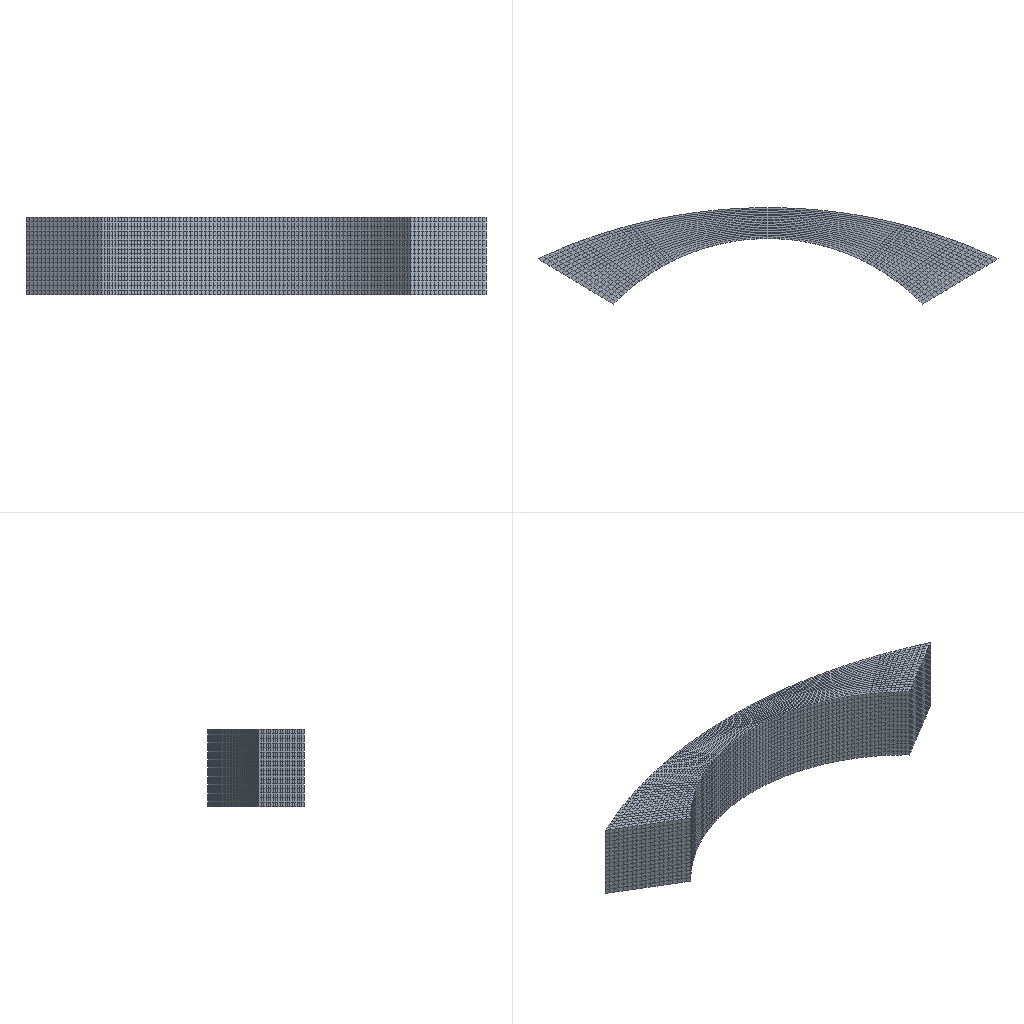Simulation study | abaqus
Set-up summary, first 263 of 10015 lines:
category,name,step,type,value,unit,region
solver,abaqus
solver,version,,,Abaqus/Standard 3DEXPERIENCE R2017x
units,not stated in the deck,,not stated
analysis,deck,,static,static
load_step,Step-1,Step-1,static,nlgeom=True
contact,interactions,,,general=0 pairs=0 ties=0
load_step,requested,,,1
mesh,nodes,,,32040
mesh,elements,,,28424
element_type,C3D8R,,solid,28424
load,load commands in deck,,count,1
bc,support commands in deck,,count,1
material,CLUST_MAT_26318,,in results
material,CLUST_MAT_26319,,in results
material,CLUST_MAT_26320,,in results
material,CLUST_MAT_26321,,in results
material,CLUST_MAT_26322,,in results
material,CLUST_MAT_26323,,in results
material,CLUST_MAT_26324,,in results
material,CLUST_MAT_26325,,in results
material,CLUST_MAT_26326,,in results
material,CLUST_MAT_26327,,in results
material,CLUST_MAT_26328,,in results
material,CLUST_MAT_26329,,in results
material,CLUST_MAT_26330,,in results
material,CLUST_MAT_26331,,in results
material,CLUST_MAT_26332,,in results
material,CLUST_MAT_26333,,in results
material,CLUST_MAT_26334,,in results
material,CLUST_MAT_26335,,in results
material,CLUST_MAT_26336,,in results
material,CLUST_MAT_26337,,in results
material,CLUST_MAT_26338,,in results
material,CLUST_MAT_26339,,in results
material,CLUST_MAT_26340,,in results
material,CLUST_MAT_26341,,in results
material,CLUST_MAT_26342,,in results
material,CLUST_MAT_26343,,in results
material,CLUST_MAT_26344,,in results
material,CLUST_MAT_26345,,in results
material,CLUST_MAT_26346,,in results
material,CLUST_MAT_26347,,in results
material,CLUST_MAT_26348,,in results
material,CLUST_MAT_26349,,in results
material,CLUST_MAT_26350,,in results
material,CLUST_MAT_26351,,in results
material,CLUST_MAT_26352,,in results
material,CLUST_MAT_26353,,in results
material,CLUST_MAT_26354,,in results
material,CLUST_MAT_26355,,in results
material,CLUST_MAT_26356,,in results
material,CLUST_MAT_26357,,in results
material,CLUST_MAT_26358,,in results
material,CLUST_MAT_26359,,in results
material,CLUST_MAT_26360,,in results
material,CLUST_MAT_26361,,in results
material,CLUST_MAT_26362,,in results
material,CLUST_MAT_26363,,in results
material,CLUST_MAT_26364,,in results
material,CLUST_MAT_26365,,in results
material,CLUST_MAT_26366,,in results
material,CLUST_MAT_26367,,in results
material,CLUST_MAT_26368,,in results
material,CLUST_MAT_26369,,in results
material,CLUST_MAT_26370,,in results
material,CLUST_MAT_26371,,in results
material,CLUST_MAT_26372,,in results
material,CLUST_MAT_26373,,in results
material,CLUST_MAT_26374,,in results
material,CLUST_MAT_26375,,in results
material,CLUST_MAT_26376,,in results
material,CLUST_MAT_26377,,in results
material,CLUST_MAT_26378,,in results
material,CLUST_MAT_26379,,in results
material,CLUST_MAT_26380,,in results
material,CLUST_MAT_26381,,in results
material,CLUST_MAT_26382,,in results
material,CLUST_MAT_26383,,in results
material,CLUST_MAT_26384,,in results
material,CLUST_MAT_26385,,in results
material,CLUST_MAT_26386,,in results
material,CLUST_MAT_26387,,in results
material,CLUST_MAT_26388,,in results
material,CLUST_MAT_26389,,in results
material,CLUST_MAT_26390,,in results
material,CLUST_MAT_26391,,in results
material,CLUST_MAT_26392,,in results
material,CLUST_MAT_26393,,in results
material,CLUST_MAT_26394,,in results
material,CLUST_MAT_26395,,in results
material,CLUST_MAT_26396,,in results
material,CLUST_MAT_26397,,in results
material,CLUST_MAT_26398,,in results
material,CLUST_MAT_26399,,in results
material,CLUST_MAT_26400,,in results
material,CLUST_MAT_26401,,in results
material,CLUST_MAT_26402,,in results
material,CLUST_MAT_26403,,in results
material,CLUST_MAT_26404,,in results
material,CLUST_MAT_26405,,in results
material,CLUST_MAT_26406,,in results
material,CLUST_MAT_26407,,in results
material,CLUST_MAT_26408,,in results
material,CLUST_MAT_26409,,in results
material,CLUST_MAT_26410,,in results
material,CLUST_MAT_26411,,in results
material,CLUST_MAT_26412,,in results
material,CLUST_MAT_26413,,in results
material,CLUST_MAT_26414,,in results
material,CLUST_MAT_26415,,in results
material,CLUST_MAT_26416,,in results
material,CLUST_MAT_26417,,in results
material,CLUST_MAT_26418,,in results
material,CLUST_MAT_26419,,in results
material,CLUST_MAT_26420,,in results
material,CLUST_MAT_26421,,in results
material,CLUST_MAT_26422,,in results
material,CLUST_MAT_26423,,in results
material,CLUST_MAT_26424,,in results
material,CLUST_MAT_26425,,in results
material,CLUST_MAT_26426,,in results
material,CLUST_MAT_26427,,in results
material,CLUST_MAT_26428,,in results
material,CLUST_MAT_26429,,in results
material,CLUST_MAT_26430,,in results
material,CLUST_MAT_26431,,in results
material,CLUST_MAT_26432,,in results
material,CLUST_MAT_26433,,in results
material,CLUST_MAT_26434,,in results
material,CLUST_MAT_26435,,in results
material,CLUST_MAT_26436,,in results
material,CLUST_MAT_26437,,in results
material,CLUST_MAT_26438,,in results
material,CLUST_MAT_26439,,in results
material,CLUST_MAT_26440,,in results
material,CLUST_MAT_26441,,in results
material,CLUST_MAT_26442,,in results
material,CLUST_MAT_26443,,in results
material,CLUST_MAT_26444,,in results
material,CLUST_MAT_26445,,in results
material,CLUST_MAT_26446,,in results
material,CLUST_MAT_26447,,in results
material,CLUST_MAT_26448,,in results
material,CLUST_MAT_26449,,in results
material,CLUST_MAT_26450,,in results
material,CLUST_MAT_26451,,in results
material,CLUST_MAT_26452,,in results
material,CLUST_MAT_26453,,in results
material,CLUST_MAT_26454,,in results
material,CLUST_MAT_26455,,in results
material,CLUST_MAT_26456,,in results
material,CLUST_MAT_26457,,in results
material,CLUST_MAT_26458,,in results
material,CLUST_MAT_26459,,in results
material,CLUST_MAT_26460,,in results
material,CLUST_MAT_26461,,in results
material,CLUST_MAT_26462,,in results
material,CLUST_MAT_26463,,in results
material,CLUST_MAT_26464,,in results
material,CLUST_MAT_26465,,in results
material,CLUST_MAT_26466,,in results
material,CLUST_MAT_26467,,in results
material,CLUST_MAT_26468,,in results
material,CLUST_MAT_26469,,in results
material,CLUST_MAT_26470,,in results
material,CLUST_MAT_26471,,in results
material,CLUST_MAT_26472,,in results
material,CLUST_MAT_26473,,in results
material,CLUST_MAT_26474,,in results
material,CLUST_MAT_26475,,in results
material,CLUST_MAT_26476,,in results
material,CLUST_MAT_26477,,in results
material,CLUST_MAT_26478,,in results
material,CLUST_MAT_26479,,in results
material,CLUST_MAT_26480,,in results
material,CLUST_MAT_26481,,in results
material,CLUST_MAT_26482,,in results
material,CLUST_MAT_26483,,in results
material,CLUST_MAT_26484,,in results
material,CLUST_MAT_26485,,in results
material,CLUST_MAT_26486,,in results
material,CLUST_MAT_26487,,in results
material,CLUST_MAT_26488,,in results
material,CLUST_MAT_26489,,in results
material,CLUST_MAT_26490,,in results
material,CLUST_MAT_26491,,in results
material,CLUST_MAT_26492,,in results
material,CLUST_MAT_26493,,in results
material,CLUST_MAT_26494,,in results
material,CLUST_MAT_26495,,in results
material,CLUST_MAT_26496,,in results
material,CLUST_MAT_26497,,in results
material,CLUST_MAT_26498,,in results
material,CLUST_MAT_26499,,in results
material,CLUST_MAT_26500,,in results
material,CLUST_MAT_26501,,in results
material,CLUST_MAT_26502,,in results
material,CLUST_MAT_26503,,in results
material,CLUST_MAT_26504,,in results
material,CLUST_MAT_26505,,in results
material,CLUST_MAT_26506,,in results
material,CLUST_MAT_26507,,in results
material,CLUST_MAT_26508,,in results
material,CLUST_MAT_26509,,in results
material,CLUST_MAT_26510,,in results
material,CLUST_MAT_26511,,in results
material,CLUST_MAT_26512,,in results
material,CLUST_MAT_26513,,in results
material,CLUST_MAT_26514,,in results
material,CLUST_MAT_26515,,in results
material,CLUST_MAT_26516,,in results
material,CLUST_MAT_26517,,in results
material,CLUST_MAT_26518,,in results
material,CLUST_MAT_26519,,in results
material,CLUST_MAT_26520,,in results
material,CLUST_MAT_26521,,in results
material,CLUST_MAT_26522,,in results
material,CLUST_MAT_26523,,in results
material,CLUST_MAT_26524,,in results
material,CLUST_MAT_26525,,in results
material,CLUST_MAT_26526,,in results
material,CLUST_MAT_26527,,in results
material,CLUST_MAT_26528,,in results
material,CLUST_MAT_26529,,in results
material,CLUST_MAT_26530,,in results
material,CLUST_MAT_26531,,in results
material,CLUST_MAT_26532,,in results
material,CLUST_MAT_26533,,in results
material,CLUST_MAT_26534,,in results
material,CLUST_MAT_26535,,in results
material,CLUST_MAT_26536,,in results
material,CLUST_MAT_26537,,in results
material,CLUST_MAT_26538,,in results
material,CLUST_MAT_26539,,in results
material,CLUST_MAT_26540,,in results
material,CLUST_MAT_26541,,in results
material,CLUST_MAT_26542,,in results
material,CLUST_MAT_26543,,in results
material,CLUST_MAT_26544,,in results
material,CLUST_MAT_26545,,in results
material,CLUST_MAT_26546,,in results
material,CLUST_MAT_26547,,in results
material,CLUST_MAT_26548,,in results
material,CLUST_MAT_26549,,in results
material,CLUST_MAT_26550,,in results
material,CLUST_MAT_26551,,in results
material,CLUST_MAT_26552,,in results
material,CLUST_MAT_26553,,in results
material,CLUST_MAT_26554,,in results
material,CLUST_MAT_26555,,in results
material,CLUST_MAT_26556,,in results
material,CLUST_MAT_26557,,in results
material,CLUST_MAT_26558,,in results
material,CLUST_MAT_26559,,in results
material,CLUST_MAT_26560,,in results
material,CLUST_MAT_26561,,in results
material,CLUST_MAT_26562,,in results
material,CLUST_MAT_26563,,in results
material,CLUST_MAT_26564,,in results
material,CLUST_MAT_26565,,in results
material,CLUST_MAT_26566,,in results
material,CLUST_MAT_26567,,in results
Abaqus input file, long lists of numbers shortened, first 1408 of 8227 lines:
**
**     _____ _ _         __  __           _ _  __ _          _
**    |  ___(_) | ___   |  \/  | ___   __| (_)/ _(_) ___  __| |
**    | |_  | | |/ _ \  | |\/| |/ _ \ / _` | | |_| |/ _ \/ _` |
**    |  _| | | |  __/  | |  | | (_) | (_| | |  _| |  __/ (_| |
**    |_|   |_|_|\___|  |_|  |_|\___/ \__,_|_|_| |_|\___|\__,_|
**
**    by SIMULIA Tosca Structure 3DEXPERIENCE R2017x Build R419 - 20161007T200008Z
**    Time: Tue Jun 06 19:57:50 2023
**
*Heading
** Job name: Opt-Process-1-Job Model name: Model-1
** Generated by: Abaqus/CAE 2017
*Preprint, echo=NO, model=NO, history=NO, contact=NO
** ----------------------------------------------------------------
**
** PART INSTANCE: Part-1-1
**
*Node
	      1,        1000.,           0.,         500.
	      2,   982.225,   18.105,         500.
** (32038 more lines like these left out)
*ELEMENT, TYPE=C3D8R, ELSET=ELSET_I_FORCE_REQ_0
	1, 1603, 1604, 1693, 1692, 1, 2, 91, 90
	2, 1604, 1605, 1694, 1693, 2, 3, 92, 91
** (28422 more lines like these left out)
*Elset, elset=_Part-1-1_ALL_ELEMENTS, generate
	     1,  28424,      1
*Nset, nset=Part-1-1_Set-1, generate
	     1,  32040,      1
*Elset, elset=Part-1-1_Set-1, generate
	     1,  28424,      1
** Section: Section-1
**
** NEW ELEMENT SET ADDED BY THE OPTIMIZATION SYSTEM
**
*ELSET, ELSET=MOD_PART-1-1_SET-1, GENERATE
	1, 88, 87
	89, 176, 87
** (305 more lines like these left out)
**
** NEW PROPERTY BASED ON PROPERTY 1 ADDED BY THE OPTIMIZATION SYSTEM
**
*SOLID SECTION, ELSET=MOD_PART-1-1_SET-1, MATERIAL=MATERIAL-1
	1.0
**
** NEW ELEMENT SET ADDED BY THE OPTIMIZATION SYSTEM
**
*ELSET, ELSET=EL_P1_M13963_1, GENERATE
	2, 3, 1
	86, 87, 1
** (42 more lines like these left out)
**
** NEW PROPERTY BASED ON PROPERTY 1 ADDED BY THE OPTIMIZATION SYSTEM
**
*SOLID SECTION, ELSET=EL_P1_M13963_1, MATERIAL=CLUST_MAT_36317
	1.0
**
** NEW ELEMENT SET ADDED BY THE OPTIMIZATION SYSTEM
**
*ELSET, ELSET=EL_P1_M12730_1, GENERATE
	4, 1412, 1408
	1493, 1493, 1408
**
** NEW PROPERTY BASED ON PROPERTY 1 ADDED BY THE OPTIMIZATION SYSTEM
**
*SOLID SECTION, ELSET=EL_P1_M12730_1, MATERIAL=CLUST_MAT_36280
	1.0
**
** NEW ELEMENT SET ADDED BY THE OPTIMIZATION SYSTEM
**
*ELSET, ELSET=EL_P1_M8508_1, GENERATE
	5, 1413, 1408
	1492, 1492, 1408
**
** NEW PROPERTY BASED ON PROPERTY 1 ADDED BY THE OPTIMIZATION SYSTEM
**
*SOLID SECTION, ELSET=EL_P1_M8508_1, MATERIAL=CLUST_MAT_36244
	1.0
**
** NEW ELEMENT SET ADDED BY THE OPTIMIZATION SYSTEM
**
*ELSET, ELSET=EL_P1_M59141_1, GENERATE
	6, 83, 77
	1414, 1491, 77
**
** NEW PROPERTY BASED ON PROPERTY 1 ADDED BY THE OPTIMIZATION SYSTEM
**
*SOLID SECTION, ELSET=EL_P1_M59141_1, MATERIAL=CLUST_MAT_36223
	1.0
**
** NEW ELEMENT SET ADDED BY THE OPTIMIZATION SYSTEM
**
*ELSET, ELSET=EL_P1_M16552_1, GENERATE
	7, 1415, 1408
	1490, 1490, 1408
**
** NEW PROPERTY BASED ON PROPERTY 1 ADDED BY THE OPTIMIZATION SYSTEM
**
*SOLID SECTION, ELSET=EL_P1_M16552_1, MATERIAL=CLUST_MAT_36202
	1.0
**
** NEW ELEMENT SET ADDED BY THE OPTIMIZATION SYSTEM
**
*ELSET, ELSET=EL_P1_M28802_1
	8, 1489
**
** NEW PROPERTY BASED ON PROPERTY 1 ADDED BY THE OPTIMIZATION SYSTEM
**
*SOLID SECTION, ELSET=EL_P1_M28802_1, MATERIAL=CLUST_MAT_36184
	1.0
**
** NEW ELEMENT SET ADDED BY THE OPTIMIZATION SYSTEM
**
*ELSET, ELSET=EL_P1_M42797_1, GENERATE
	9, 1417, 1408
	1488, 1488, 1408
**
** NEW PROPERTY BASED ON PROPERTY 1 ADDED BY THE OPTIMIZATION SYSTEM
**
*SOLID SECTION, ELSET=EL_P1_M42797_1, MATERIAL=CLUST_MAT_36134
	1.0
**
** NEW ELEMENT SET ADDED BY THE OPTIMIZATION SYSTEM
**
*ELSET, ELSET=EL_P1_M25813_1, GENERATE
	10, 1418, 1408
	1487, 1487, 1408
**
** NEW PROPERTY BASED ON PROPERTY 1 ADDED BY THE OPTIMIZATION SYSTEM
**
*SOLID SECTION, ELSET=EL_P1_M25813_1, MATERIAL=CLUST_MAT_36089
	1.0
**
** NEW ELEMENT SET ADDED BY THE OPTIMIZATION SYSTEM
**
*ELSET, ELSET=EL_P1_M27718_1, GENERATE
	11, 78, 67
	1419, 1486, 67
**
** NEW PROPERTY BASED ON PROPERTY 1 ADDED BY THE OPTIMIZATION SYSTEM
**
*SOLID SECTION, ELSET=EL_P1_M27718_1, MATERIAL=CLUST_MAT_36044
	1.0
**
** NEW ELEMENT SET ADDED BY THE OPTIMIZATION SYSTEM
**
*ELSET, ELSET=EL_P1_M60534_1
	12, 1420
**
** NEW PROPERTY BASED ON PROPERTY 1 ADDED BY THE OPTIMIZATION SYSTEM
**
*SOLID SECTION, ELSET=EL_P1_M60534_1, MATERIAL=CLUST_MAT_36002
	1.0
**
** NEW ELEMENT SET ADDED BY THE OPTIMIZATION SYSTEM
**
*ELSET, ELSET=EL_P1_M21999_1, GENERATE
	13, 76, 63
	1421, 1484, 63
**
** NEW PROPERTY BASED ON PROPERTY 1 ADDED BY THE OPTIMIZATION SYSTEM
**
*SOLID SECTION, ELSET=EL_P1_M21999_1, MATERIAL=CLUST_MAT_35954
	1.0
**
** NEW ELEMENT SET ADDED BY THE OPTIMIZATION SYSTEM
**
*ELSET, ELSET=EL_P1_M44446_1
	14, 1483
**
** NEW PROPERTY BASED ON PROPERTY 1 ADDED BY THE OPTIMIZATION SYSTEM
**
*SOLID SECTION, ELSET=EL_P1_M44446_1, MATERIAL=CLUST_MAT_35937
	1.0
**
** NEW ELEMENT SET ADDED BY THE OPTIMIZATION SYSTEM
**
*ELSET, ELSET=EL_P1_M31457_1
	15, 1482
**
** NEW PROPERTY BASED ON PROPERTY 1 ADDED BY THE OPTIMIZATION SYSTEM
**
*SOLID SECTION, ELSET=EL_P1_M31457_1, MATERIAL=CLUST_MAT_35900
	1.0
**
** NEW ELEMENT SET ADDED BY THE OPTIMIZATION SYSTEM
**
*ELSET, ELSET=EL_P1_M17032_1
	16, 1481
**
** NEW PROPERTY BASED ON PROPERTY 1 ADDED BY THE OPTIMIZATION SYSTEM
**
*SOLID SECTION, ELSET=EL_P1_M17032_1, MATERIAL=CLUST_MAT_35864
	1.0
**
** NEW ELEMENT SET ADDED BY THE OPTIMIZATION SYSTEM
**
*ELSET, ELSET=EL_P1_M27205_1, GENERATE
	17, 72, 55
	1425, 1425, 55
**
** NEW PROPERTY BASED ON PROPERTY 1 ADDED BY THE OPTIMIZATION SYSTEM
**
*SOLID SECTION, ELSET=EL_P1_M27205_1, MATERIAL=CLUST_MAT_35808
	1.0
**
** NEW ELEMENT SET ADDED BY THE OPTIMIZATION SYSTEM
**
*ELSET, ELSET=EL_P1_M19720_1, GENERATE
	18, 71, 53
	1426, 1479, 53
**
** NEW PROPERTY BASED ON PROPERTY 1 ADDED BY THE OPTIMIZATION SYSTEM
**
*SOLID SECTION, ELSET=EL_P1_M19720_1, MATERIAL=CLUST_MAT_35768
	1.0
**
** NEW ELEMENT SET ADDED BY THE OPTIMIZATION SYSTEM
**
*ELSET, ELSET=EL_P1_M60548_1, GENERATE
	19, 70, 51
	1427, 1478, 51
**
** NEW PROPERTY BASED ON PROPERTY 1 ADDED BY THE OPTIMIZATION SYSTEM
**
*SOLID SECTION, ELSET=EL_P1_M60548_1, MATERIAL=CLUST_MAT_35697
	1.0
**
** NEW ELEMENT SET ADDED BY THE OPTIMIZATION SYSTEM
**
*ELSET, ELSET=EL_P1_M38085_1, GENERATE
	20, 69, 49
	1428, 1477, 49
**
** NEW PROPERTY BASED ON PROPERTY 1 ADDED BY THE OPTIMIZATION SYSTEM
**
*SOLID SECTION, ELSET=EL_P1_M38085_1, MATERIAL=CLUST_MAT_35596
	1.0
**
** NEW ELEMENT SET ADDED BY THE OPTIMIZATION SYSTEM
**
*ELSET, ELSET=EL_P1_M63393_1, GENERATE
	21, 68, 47
	1429, 1476, 47
**
** NEW PROPERTY BASED ON PROPERTY 1 ADDED BY THE OPTIMIZATION SYSTEM
**
*SOLID SECTION, ELSET=EL_P1_M63393_1, MATERIAL=CLUST_MAT_35491
	1.0
**
** NEW ELEMENT SET ADDED BY THE OPTIMIZATION SYSTEM
**
*ELSET, ELSET=EL_P1_M1667_1
	22, 1430
**
** NEW PROPERTY BASED ON PROPERTY 1 ADDED BY THE OPTIMIZATION SYSTEM
**
*SOLID SECTION, ELSET=EL_P1_M1667_1, MATERIAL=CLUST_MAT_35359
	1.0
**
** NEW ELEMENT SET ADDED BY THE OPTIMIZATION SYSTEM
**
*ELSET, ELSET=EL_P1_M51066_1
	23
**
** NEW PROPERTY BASED ON PROPERTY 1 ADDED BY THE OPTIMIZATION SYSTEM
**
*SOLID SECTION, ELSET=EL_P1_M51066_1, MATERIAL=CLUST_MAT_35108
	1.0
**
** NEW ELEMENT SET ADDED BY THE OPTIMIZATION SYSTEM
**
*ELSET, ELSET=EL_P1_M13452_1, GENERATE
	24, 1432, 1408
	1473, 1473, 1408
**
** NEW PROPERTY BASED ON PROPERTY 1 ADDED BY THE OPTIMIZATION SYSTEM
**
*SOLID SECTION, ELSET=EL_P1_M13452_1, MATERIAL=CLUST_MAT_34805
	1.0
**
** NEW ELEMENT SET ADDED BY THE OPTIMIZATION SYSTEM
**
*ELSET, ELSET=EL_P1_M56171_1, GENERATE
	25, 1433, 1408
	1472, 1472, 1408
**
** NEW PROPERTY BASED ON PROPERTY 1 ADDED BY THE OPTIMIZATION SYSTEM
**
*SOLID SECTION, ELSET=EL_P1_M56171_1, MATERIAL=CLUST_MAT_33849
	1.0
**
** NEW ELEMENT SET ADDED BY THE OPTIMIZATION SYSTEM
**
*ELSET, ELSET=EL_P1_M24159_1
	26, 63
**
** NEW PROPERTY BASED ON PROPERTY 1 ADDED BY THE OPTIMIZATION SYSTEM
**
*SOLID SECTION, ELSET=EL_P1_M24159_1, MATERIAL=CLUST_MAT_32665
	1.0
**
** NEW ELEMENT SET ADDED BY THE OPTIMIZATION SYSTEM
**
*ELSET, ELSET=EL_P1_M63107_1, GENERATE
	27, 62, 35
	1435, 1470, 35
**
** NEW PROPERTY BASED ON PROPERTY 1 ADDED BY THE OPTIMIZATION SYSTEM
**
*SOLID SECTION, ELSET=EL_P1_M63107_1, MATERIAL=CLUST_MAT_31641
	1.0
**
** NEW ELEMENT SET ADDED BY THE OPTIMIZATION SYSTEM
**
*ELSET, ELSET=EL_P1_M3558_1, GENERATE
	28, 61, 33
	1436, 1469, 33
**
** NEW PROPERTY BASED ON PROPERTY 1 ADDED BY THE OPTIMIZATION SYSTEM
**
*SOLID SECTION, ELSET=EL_P1_M3558_1, MATERIAL=CLUST_MAT_30077
	1.0
**
** NEW ELEMENT SET ADDED BY THE OPTIMIZATION SYSTEM
**
*ELSET, ELSET=EL_P1_M51260_1, GENERATE
	29, 60, 31
	1437, 1468, 31
**
** NEW PROPERTY BASED ON PROPERTY 1 ADDED BY THE OPTIMIZATION SYSTEM
**
*SOLID SECTION, ELSET=EL_P1_M51260_1, MATERIAL=CLUST_MAT_28696
	1.0
**
** NEW ELEMENT SET ADDED BY THE OPTIMIZATION SYSTEM
**
*ELSET, ELSET=EL_P1_M39577_1, GENERATE
	30, 59, 29
	1438, 1467, 29
**
** NEW PROPERTY BASED ON PROPERTY 1 ADDED BY THE OPTIMIZATION SYSTEM
**
*SOLID SECTION, ELSET=EL_P1_M39577_1, MATERIAL=CLUST_MAT_27613
	1.0
**
** NEW ELEMENT SET ADDED BY THE OPTIMIZATION SYSTEM
**
*ELSET, ELSET=EL_P1_M28491_1, GENERATE
	31, 58, 27
	1439, 1466, 27
**
** NEW PROPERTY BASED ON PROPERTY 1 ADDED BY THE OPTIMIZATION SYSTEM
**
*SOLID SECTION, ELSET=EL_P1_M28491_1, MATERIAL=CLUST_MAT_27002
	1.0
**
** NEW ELEMENT SET ADDED BY THE OPTIMIZATION SYSTEM
**
*ELSET, ELSET=EL_P1_M30126_1, GENERATE
	32, 57, 25
	1440, 1465, 25
**
** NEW PROPERTY BASED ON PROPERTY 1 ADDED BY THE OPTIMIZATION SYSTEM
**
*SOLID SECTION, ELSET=EL_P1_M30126_1, MATERIAL=CLUST_MAT_26674
	1.0
**
** NEW ELEMENT SET ADDED BY THE OPTIMIZATION SYSTEM
**
*ELSET, ELSET=EL_P1_M35899_1, GENERATE
	33, 1441, 1408
	1464, 1464, 1408
**
** NEW PROPERTY BASED ON PROPERTY 1 ADDED BY THE OPTIMIZATION SYSTEM
**
*SOLID SECTION, ELSET=EL_P1_M35899_1, MATERIAL=CLUST_MAT_26503
	1.0
**
** NEW ELEMENT SET ADDED BY THE OPTIMIZATION SYSTEM
**
*ELSET, ELSET=EL_P1_M19154_1
	34
**
** NEW PROPERTY BASED ON PROPERTY 1 ADDED BY THE OPTIMIZATION SYSTEM
**
*SOLID SECTION, ELSET=EL_P1_M19154_1, MATERIAL=CLUST_MAT_26447
	1.0
**
** NEW ELEMENT SET ADDED BY THE OPTIMIZATION SYSTEM
**
*ELSET, ELSET=EL_P1_M15814_1, GENERATE
	35, 54, 19
	1443, 1462, 19
**
** NEW PROPERTY BASED ON PROPERTY 1 ADDED BY THE OPTIMIZATION SYSTEM
**
*SOLID SECTION, ELSET=EL_P1_M15814_1, MATERIAL=CLUST_MAT_27675
	1.0
**
** NEW ELEMENT SET ADDED BY THE OPTIMIZATION SYSTEM
**
*ELSET, ELSET=EL_P1_M23475_1, GENERATE
	36, 1444, 1408
	1461, 1461, 1408
**
** NEW PROPERTY BASED ON PROPERTY 1 ADDED BY THE OPTIMIZATION SYSTEM
**
*SOLID SECTION, ELSET=EL_P1_M23475_1, MATERIAL=CLUST_MAT_27811
	1.0
**
** NEW ELEMENT SET ADDED BY THE OPTIMIZATION SYSTEM
**
*ELSET, ELSET=EL_P1_M62036_1, GENERATE
	37, 52, 15
	1445, 1460, 15
**
** NEW PROPERTY BASED ON PROPERTY 1 ADDED BY THE OPTIMIZATION SYSTEM
**
*SOLID SECTION, ELSET=EL_P1_M62036_1, MATERIAL=CLUST_MAT_29400
	1.0
**
** NEW ELEMENT SET ADDED BY THE OPTIMIZATION SYSTEM
**
*ELSET, ELSET=EL_P1_M37079_1, GENERATE
	38, 51, 13
	1446, 1459, 13
**
** NEW PROPERTY BASED ON PROPERTY 1 ADDED BY THE OPTIMIZATION SYSTEM
**
*SOLID SECTION, ELSET=EL_P1_M37079_1, MATERIAL=CLUST_MAT_30903
	1.0
**
** NEW ELEMENT SET ADDED BY THE OPTIMIZATION SYSTEM
**
*ELSET, ELSET=EL_P1_M44734_1, GENERATE
	39, 50, 11
	1447, 1458, 11
**
** NEW PROPERTY BASED ON PROPERTY 1 ADDED BY THE OPTIMIZATION SYSTEM
**
*SOLID SECTION, ELSET=EL_P1_M44734_1, MATERIAL=CLUST_MAT_31705
	1.0
**
** NEW ELEMENT SET ADDED BY THE OPTIMIZATION SYSTEM
**
*ELSET, ELSET=EL_P1_M16971_1
	40, 49
**
** NEW PROPERTY BASED ON PROPERTY 1 ADDED BY THE OPTIMIZATION SYSTEM
**
*SOLID SECTION, ELSET=EL_P1_M16971_1, MATERIAL=CLUST_MAT_32302
	1.0
**
** NEW ELEMENT SET ADDED BY THE OPTIMIZATION SYSTEM
**
*ELSET, ELSET=EL_P1_M54474_1, GENERATE
	41, 48, 7
	1449, 1456, 7
**
** NEW PROPERTY BASED ON PROPERTY 1 ADDED BY THE OPTIMIZATION SYSTEM
**
*SOLID SECTION, ELSET=EL_P1_M54474_1, MATERIAL=CLUST_MAT_32783
	1.0
**
** NEW ELEMENT SET ADDED BY THE OPTIMIZATION SYSTEM
**
*ELSET, ELSET=EL_P1_M40849_1, GENERATE
	42, 47, 5
	1455, 1455, 5
**
** NEW PROPERTY BASED ON PROPERTY 1 ADDED BY THE OPTIMIZATION SYSTEM
**
*SOLID SECTION, ELSET=EL_P1_M40849_1, MATERIAL=CLUST_MAT_33163
	1.0
**
** NEW ELEMENT SET ADDED BY THE OPTIMIZATION SYSTEM
**
*ELSET, ELSET=EL_P1_M60818_1, GENERATE
	43, 46, 3
	1451, 1454, 3
**
** NEW PROPERTY BASED ON PROPERTY 1 ADDED BY THE OPTIMIZATION SYSTEM
**
*SOLID SECTION, ELSET=EL_P1_M60818_1, MATERIAL=CLUST_MAT_33540
	1.0
**
** NEW ELEMENT SET ADDED BY THE OPTIMIZATION SYSTEM
**
*ELSET, ELSET=EL_P1_M64724_1, GENERATE
	44, 45, 1
	1452, 1453, 1
**
** NEW PROPERTY BASED ON PROPERTY 1 ADDED BY THE OPTIMIZATION SYSTEM
**
*SOLID SECTION, ELSET=EL_P1_M64724_1, MATERIAL=CLUST_MAT_33714
	1.0
**
** NEW ELEMENT SET ADDED BY THE OPTIMIZATION SYSTEM
**
*ELSET, ELSET=EL_P1_M15574_1
	53
**
** NEW PROPERTY BASED ON PROPERTY 1 ADDED BY THE OPTIMIZATION SYSTEM
**
*SOLID SECTION, ELSET=EL_P1_M15574_1, MATERIAL=CLUST_MAT_27810
	1.0
**
** NEW ELEMENT SET ADDED BY THE OPTIMIZATION SYSTEM
**
*ELSET, ELSET=EL_P1_M3355_1, GENERATE
	55, 1442, 1387
	1463, 1463, 1387
**
** NEW PROPERTY BASED ON PROPERTY 1 ADDED BY THE OPTIMIZATION SYSTEM
**
*SOLID SECTION, ELSET=EL_P1_M3355_1, MATERIAL=CLUST_MAT_26448
	1.0
**
** NEW ELEMENT SET ADDED BY THE OPTIMIZATION SYSTEM
**
*ELSET, ELSET=EL_P1_M60254_1
	56
**
** NEW PROPERTY BASED ON PROPERTY 1 ADDED BY THE OPTIMIZATION SYSTEM
**
*SOLID SECTION, ELSET=EL_P1_M60254_1, MATERIAL=CLUST_MAT_26502
	1.0
**
** NEW ELEMENT SET ADDED BY THE OPTIMIZATION SYSTEM
**
*ELSET, ELSET=EL_P1_M48142_1
	64
**
** NEW PROPERTY BASED ON PROPERTY 1 ADDED BY THE OPTIMIZATION SYSTEM
**
*SOLID SECTION, ELSET=EL_P1_M48142_1, MATERIAL=CLUST_MAT_33848
	1.0
**
** NEW ELEMENT SET ADDED BY THE OPTIMIZATION SYSTEM
**
*ELSET, ELSET=EL_P1_M21481_1
	65
**
** NEW PROPERTY BASED ON PROPERTY 1 ADDED BY THE OPTIMIZATION SYSTEM
**
*SOLID SECTION, ELSET=EL_P1_M21481_1, MATERIAL=CLUST_MAT_34804
	1.0
**
** NEW ELEMENT SET ADDED BY THE OPTIMIZATION SYSTEM
**
*ELSET, ELSET=EL_P1_M65475_1, GENERATE
	66, 1431, 1365
	1474, 1474, 1365
**
** NEW PROPERTY BASED ON PROPERTY 1 ADDED BY THE OPTIMIZATION SYSTEM
**
*SOLID SECTION, ELSET=EL_P1_M65475_1, MATERIAL=CLUST_MAT_35107
	1.0
**
** NEW ELEMENT SET ADDED BY THE OPTIMIZATION SYSTEM
**
*ELSET, ELSET=EL_P1_M25062_1
	67, 1475
**
** NEW PROPERTY BASED ON PROPERTY 1 ADDED BY THE OPTIMIZATION SYSTEM
**
*SOLID SECTION, ELSET=EL_P1_M25062_1, MATERIAL=CLUST_MAT_35358
	1.0
**
** NEW ELEMENT SET ADDED BY THE OPTIMIZATION SYSTEM
**
*ELSET, ELSET=EL_P1_M21214_1
	73, 1424
**
** NEW PROPERTY BASED ON PROPERTY 1 ADDED BY THE OPTIMIZATION SYSTEM
**
*SOLID SECTION, ELSET=EL_P1_M21214_1, MATERIAL=CLUST_MAT_35863
	1.0
**
** NEW ELEMENT SET ADDED BY THE OPTIMIZATION SYSTEM
**
*ELSET, ELSET=EL_P1_M16984_1
	74, 1423
**
** NEW PROPERTY BASED ON PROPERTY 1 ADDED BY THE OPTIMIZATION SYSTEM
**
*SOLID SECTION, ELSET=EL_P1_M16984_1, MATERIAL=CLUST_MAT_35899
	1.0
**
** NEW ELEMENT SET ADDED BY THE OPTIMIZATION SYSTEM
**
*ELSET, ELSET=EL_P1_M51963_1
	75, 1422
**
** NEW PROPERTY BASED ON PROPERTY 1 ADDED BY THE OPTIMIZATION SYSTEM
**
*SOLID SECTION, ELSET=EL_P1_M51963_1, MATERIAL=CLUST_MAT_35936
	1.0
**
** NEW ELEMENT SET ADDED BY THE OPTIMIZATION SYSTEM
**
*ELSET, ELSET=EL_P1_M17304_1
	77, 1485
**
** NEW PROPERTY BASED ON PROPERTY 1 ADDED BY THE OPTIMIZATION SYSTEM
**
*SOLID SECTION, ELSET=EL_P1_M17304_1, MATERIAL=CLUST_MAT_36001
	1.0
**
** NEW ELEMENT SET ADDED BY THE OPTIMIZATION SYSTEM
**
*ELSET, ELSET=EL_P1_M944_1
	79
**
** NEW PROPERTY BASED ON PROPERTY 1 ADDED BY THE OPTIMIZATION SYSTEM
**
*SOLID SECTION, ELSET=EL_P1_M944_1, MATERIAL=CLUST_MAT_36088
	1.0
**
** NEW ELEMENT SET ADDED BY THE OPTIMIZATION SYSTEM
**
*ELSET, ELSET=EL_P1_M2243_1
	80
**
** NEW PROPERTY BASED ON PROPERTY 1 ADDED BY THE OPTIMIZATION SYSTEM
**
*SOLID SECTION, ELSET=EL_P1_M2243_1, MATERIAL=CLUST_MAT_36133
	1.0
**
** NEW ELEMENT SET ADDED BY THE OPTIMIZATION SYSTEM
**
*ELSET, ELSET=EL_P1_M24788_1
	81, 1416
**
** NEW PROPERTY BASED ON PROPERTY 1 ADDED BY THE OPTIMIZATION SYSTEM
**
*SOLID SECTION, ELSET=EL_P1_M24788_1, MATERIAL=CLUST_MAT_36183
	1.0
**
** NEW ELEMENT SET ADDED BY THE OPTIMIZATION SYSTEM
**
*ELSET, ELSET=EL_P1_M61254_1
	82
**
** NEW PROPERTY BASED ON PROPERTY 1 ADDED BY THE OPTIMIZATION SYSTEM
**
*SOLID SECTION, ELSET=EL_P1_M61254_1, MATERIAL=CLUST_MAT_36201
	1.0
**
** NEW ELEMENT SET ADDED BY THE OPTIMIZATION SYSTEM
**
*ELSET, ELSET=EL_P1_M6533_1
	84
**
** NEW PROPERTY BASED ON PROPERTY 1 ADDED BY THE OPTIMIZATION SYSTEM
**
*SOLID SECTION, ELSET=EL_P1_M6533_1, MATERIAL=CLUST_MAT_36243
	1.0
**
** NEW ELEMENT SET ADDED BY THE OPTIMIZATION SYSTEM
**
*ELSET, ELSET=EL_P1_M8684_1
	85
**
** NEW PROPERTY BASED ON PROPERTY 1 ADDED BY THE OPTIMIZATION SYSTEM
**
*SOLID SECTION, ELSET=EL_P1_M8684_1, MATERIAL=CLUST_MAT_36279
	1.0
**
** NEW ELEMENT SET ADDED BY THE OPTIMIZATION SYSTEM
**
*ELSET, ELSET=EL_P1_M45450_1
	92
**
** NEW PROPERTY BASED ON PROPERTY 1 ADDED BY THE OPTIMIZATION SYSTEM
**
*SOLID SECTION, ELSET=EL_P1_M45450_1, MATERIAL=CLUST_MAT_36310
	1.0
**
** NEW ELEMENT SET ADDED BY THE OPTIMIZATION SYSTEM
**
*ELSET, ELSET=EL_P1_M59751_1
	93, 172
**
** NEW PROPERTY BASED ON PROPERTY 1 ADDED BY THE OPTIMIZATION SYSTEM
**
*SOLID SECTION, ELSET=EL_P1_M59751_1, MATERIAL=CLUST_MAT_36277
	1.0
**
** NEW ELEMENT SET ADDED BY THE OPTIMIZATION SYSTEM
**
*ELSET, ELSET=EL_P1_M18009_1, GENERATE
	94, 1326, 1232
	1403, 1403, 1232
**
** NEW PROPERTY BASED ON PROPERTY 1 ADDED BY THE OPTIMIZATION SYSTEM
**
*SOLID SECTION, ELSET=EL_P1_M18009_1, MATERIAL=CLUST_MAT_36245
	1.0
**
** NEW ELEMENT SET ADDED BY THE OPTIMIZATION SYSTEM
**
*ELSET, ELSET=EL_P1_M10623_1, GENERATE
	95, 170, 75
	1327, 1402, 75
**
** NEW PROPERTY BASED ON PROPERTY 1 ADDED BY THE OPTIMIZATION SYSTEM
**
*SOLID SECTION, ELSET=EL_P1_M10623_1, MATERIAL=CLUST_MAT_36226
	1.0
**
** NEW ELEMENT SET ADDED BY THE OPTIMIZATION SYSTEM
**
*ELSET, ELSET=EL_P1_M45210_1
	96, 1328
**
** NEW PROPERTY BASED ON PROPERTY 1 ADDED BY THE OPTIMIZATION SYSTEM
**
*SOLID SECTION, ELSET=EL_P1_M45210_1, MATERIAL=CLUST_MAT_36207
	1.0
**
** NEW ELEMENT SET ADDED BY THE OPTIMIZATION SYSTEM
**
*ELSET, ELSET=EL_P1_M26695_1
	97, 1329
**
** NEW PROPERTY BASED ON PROPERTY 1 ADDED BY THE OPTIMIZATION SYSTEM
**
*SOLID SECTION, ELSET=EL_P1_M26695_1, MATERIAL=CLUST_MAT_36194
	1.0
**
** NEW ELEMENT SET ADDED BY THE OPTIMIZATION SYSTEM
**
*ELSET, ELSET=EL_P1_M44910_1, GENERATE
	98, 1330, 1232
	1399, 1399, 1232
**
** NEW PROPERTY BASED ON PROPERTY 1 ADDED BY THE OPTIMIZATION SYSTEM
**
*SOLID SECTION, ELSET=EL_P1_M44910_1, MATERIAL=CLUST_MAT_36144
	1.0
**
** NEW ELEMENT SET ADDED BY THE OPTIMIZATION SYSTEM
**
*ELSET, ELSET=EL_P1_M29827_1, GENERATE
	99, 166, 67
	1331, 1398, 67
**
** NEW PROPERTY BASED ON PROPERTY 1 ADDED BY THE OPTIMIZATION SYSTEM
**
*SOLID SECTION, ELSET=EL_P1_M29827_1, MATERIAL=CLUST_MAT_36086
	1.0
**
** NEW ELEMENT SET ADDED BY THE OPTIMIZATION SYSTEM
**
*ELSET, ELSET=EL_P1_M54270_1, GENERATE
	100, 165, 65
	1332, 1397, 65
**
** NEW PROPERTY BASED ON PROPERTY 1 ADDED BY THE OPTIMIZATION SYSTEM
**
*SOLID SECTION, ELSET=EL_P1_M54270_1, MATERIAL=CLUST_MAT_36032
	1.0
**
** NEW ELEMENT SET ADDED BY THE OPTIMIZATION SYSTEM
**
*ELSET, ELSET=EL_P1_M47929_1, GENERATE
	101, 164, 63
	1333, 1396, 63
**
** NEW PROPERTY BASED ON PROPERTY 1 ADDED BY THE OPTIMIZATION SYSTEM
**
*SOLID SECTION, ELSET=EL_P1_M47929_1, MATERIAL=CLUST_MAT_35985
	1.0
**
** NEW ELEMENT SET ADDED BY THE OPTIMIZATION SYSTEM
**
*ELSET, ELSET=EL_P1_M4646_1
	102, 1395
**
** NEW PROPERTY BASED ON PROPERTY 1 ADDED BY THE OPTIMIZATION SYSTEM
**
*SOLID SECTION, ELSET=EL_P1_M4646_1, MATERIAL=CLUST_MAT_35949
	1.0
**
** NEW ELEMENT SET ADDED BY THE OPTIMIZATION SYSTEM
**
*ELSET, ELSET=EL_P1_M38391_1
	103, 1394
**
** NEW PROPERTY BASED ON PROPERTY 1 ADDED BY THE OPTIMIZATION SYSTEM
**
*SOLID SECTION, ELSET=EL_P1_M38391_1, MATERIAL=CLUST_MAT_35909
	1.0
**
** NEW ELEMENT SET ADDED BY THE OPTIMIZATION SYSTEM
**
*ELSET, ELSET=EL_P1_M7508_1
	104
**
** NEW PROPERTY BASED ON PROPERTY 1 ADDED BY THE OPTIMIZATION SYSTEM
**
*SOLID SECTION, ELSET=EL_P1_M7508_1, MATERIAL=CLUST_MAT_35870
	1.0
**
** NEW ELEMENT SET ADDED BY THE OPTIMIZATION SYSTEM
**
*ELSET, ELSET=EL_P1_M62801_1, GENERATE
	105, 160, 55
	1337, 1392, 55
**
** NEW PROPERTY BASED ON PROPERTY 1 ADDED BY THE OPTIMIZATION SYSTEM
**
*SOLID SECTION, ELSET=EL_P1_M62801_1, MATERIAL=CLUST_MAT_35826
	1.0
**
** NEW ELEMENT SET ADDED BY THE OPTIMIZATION SYSTEM
**
*ELSET, ELSET=EL_P1_M64962_1, GENERATE
	106, 159, 53
	1391, 1391, 53
**
** NEW PROPERTY BASED ON PROPERTY 1 ADDED BY THE OPTIMIZATION SYSTEM
**
*SOLID SECTION, ELSET=EL_P1_M64962_1, MATERIAL=CLUST_MAT_35783
	1.0
**
** NEW ELEMENT SET ADDED BY THE OPTIMIZATION SYSTEM
**
*ELSET, ELSET=EL_P1_M40262_1
	107, 158
**
** NEW PROPERTY BASED ON PROPERTY 1 ADDED BY THE OPTIMIZATION SYSTEM
**
*SOLID SECTION, ELSET=EL_P1_M40262_1, MATERIAL=CLUST_MAT_35712
	1.0
**
** NEW ELEMENT SET ADDED BY THE OPTIMIZATION SYSTEM
**
*ELSET, ELSET=EL_P1_M54028_1, GENERATE
	108, 157, 49
	1389, 1389, 49
**
** NEW PROPERTY BASED ON PROPERTY 1 ADDED BY THE OPTIMIZATION SYSTEM
**
*SOLID SECTION, ELSET=EL_P1_M54028_1, MATERIAL=CLUST_MAT_35603
	1.0
**
** NEW ELEMENT SET ADDED BY THE OPTIMIZATION SYSTEM
**
*ELSET, ELSET=EL_P1_M53016_1, GENERATE
	109, 156, 47
	1341, 1341, 47
**
** NEW PROPERTY BASED ON PROPERTY 1 ADDED BY THE OPTIMIZATION SYSTEM
**
*SOLID SECTION, ELSET=EL_P1_M53016_1, MATERIAL=CLUST_MAT_35492
	1.0
**
** NEW ELEMENT SET ADDED BY THE OPTIMIZATION SYSTEM
**
*ELSET, ELSET=EL_P1_M43373_1
	110
**
** NEW PROPERTY BASED ON PROPERTY 1 ADDED BY THE OPTIMIZATION SYSTEM
**
*SOLID SECTION, ELSET=EL_P1_M43373_1, MATERIAL=CLUST_MAT_35356
	1.0
**
** NEW ELEMENT SET ADDED BY THE OPTIMIZATION SYSTEM
**
*ELSET, ELSET=EL_P1_M59142_1
	111, 154
**
** NEW PROPERTY BASED ON PROPERTY 1 ADDED BY THE OPTIMIZATION SYSTEM
**
*SOLID SECTION, ELSET=EL_P1_M59142_1, MATERIAL=CLUST_MAT_35097
	1.0
**
** NEW ELEMENT SET ADDED BY THE OPTIMIZATION SYSTEM
**
*ELSET, ELSET=EL_P1_M19244_1
	112
**
** NEW PROPERTY BASED ON PROPERTY 1 ADDED BY THE OPTIMIZATION SYSTEM
**
*SOLID SECTION, ELSET=EL_P1_M19244_1, MATERIAL=CLUST_MAT_34766
	1.0
**
** NEW ELEMENT SET ADDED BY THE OPTIMIZATION SYSTEM
**
*ELSET, ELSET=EL_P1_M58322_1, GENERATE
	113, 152, 39
	1345, 1384, 39
**
** NEW PROPERTY BASED ON PROPERTY 1 ADDED BY THE OPTIMIZATION SYSTEM
**
*SOLID SECTION, ELSET=EL_P1_M58322_1, MATERIAL=CLUST_MAT_33854
	1.0
**
** NEW ELEMENT SET ADDED BY THE OPTIMIZATION SYSTEM
**
*ELSET, ELSET=EL_P1_M59764_1, GENERATE
	114, 151, 37
	1346, 1383, 37
**
** NEW PROPERTY BASED ON PROPERTY 1 ADDED BY THE OPTIMIZATION SYSTEM
**
*SOLID SECTION, ELSET=EL_P1_M59764_1, MATERIAL=CLUST_MAT_32672
	1.0
**
** NEW ELEMENT SET ADDED BY THE OPTIMIZATION SYSTEM
**
*ELSET, ELSET=EL_P1_M59767_1
	115
**
** NEW PROPERTY BASED ON PROPERTY 1 ADDED BY THE OPTIMIZATION SYSTEM
**
*SOLID SECTION, ELSET=EL_P1_M59767_1, MATERIAL=CLUST_MAT_31686
	1.0
**
** NEW ELEMENT SET ADDED BY THE OPTIMIZATION SYSTEM
**
*ELSET, ELSET=EL_P1_M48333_1
	116, 1381
**
** NEW PROPERTY BASED ON PROPERTY 1 ADDED BY THE OPTIMIZATION SYSTEM
**
*SOLID SECTION, ELSET=EL_P1_M48333_1, MATERIAL=CLUST_MAT_30222
	1.0
**
** NEW ELEMENT SET ADDED BY THE OPTIMIZATION SYSTEM
**
*ELSET, ELSET=EL_P1_M27264_1
	117, 1380
**
** NEW PROPERTY BASED ON PROPERTY 1 ADDED BY THE OPTIMIZATION SYSTEM
**
*SOLID SECTION, ELSET=EL_P1_M27264_1, MATERIAL=CLUST_MAT_28954
	1.0
**
** NEW ELEMENT SET ADDED BY THE OPTIMIZATION SYSTEM
**
*ELSET, ELSET=EL_P1_M25354_1, GENERATE
	118, 147, 29
	1350, 1379, 29
**
** NEW PROPERTY BASED ON PROPERTY 1 ADDED BY THE OPTIMIZATION SYSTEM
**
*SOLID SECTION, ELSET=EL_P1_M25354_1, MATERIAL=CLUST_MAT_27812
	1.0
**
** NEW ELEMENT SET ADDED BY THE OPTIMIZATION SYSTEM
**
*ELSET, ELSET=EL_P1_M43395_1, GENERATE
	119, 146, 27
	1351, 1351, 27
**
** NEW PROPERTY BASED ON PROPERTY 1 ADDED BY THE OPTIMIZATION SYSTEM
**
*SOLID SECTION, ELSET=EL_P1_M43395_1, MATERIAL=CLUST_MAT_27172
	1.0
**
** NEW ELEMENT SET ADDED BY THE OPTIMIZATION SYSTEM
**
*ELSET, ELSET=EL_P1_M13462_1
	120
**
** NEW PROPERTY BASED ON PROPERTY 1 ADDED BY THE OPTIMIZATION SYSTEM
**
*SOLID SECTION, ELSET=EL_P1_M13462_1, MATERIAL=CLUST_MAT_26834
	1.0
**
** NEW ELEMENT SET ADDED BY THE OPTIMIZATION SYSTEM
**
*ELSET, ELSET=EL_P1_M43942_1
	121, 144
**
** NEW PROPERTY BASED ON PROPERTY 1 ADDED BY THE OPTIMIZATION SYSTEM
**
*SOLID SECTION, ELSET=EL_P1_M43942_1, MATERIAL=CLUST_MAT_26620
	1.0
**
** NEW ELEMENT SET ADDED BY THE OPTIMIZATION SYSTEM
**
*ELSET, ELSET=EL_P1_M60302_1
	122, 1354
**
** NEW PROPERTY BASED ON PROPERTY 1 ADDED BY THE OPTIMIZATION SYSTEM
**
*SOLID SECTION, ELSET=EL_P1_M60302_1, MATERIAL=CLUST_MAT_26533
	1.0
**
** NEW ELEMENT SET ADDED BY THE OPTIMIZATION SYSTEM
**
*ELSET, ELSET=EL_P1_M41922_1
	123
**
** NEW PROPERTY BASED ON PROPERTY 1 ADDED BY THE OPTIMIZATION SYSTEM
**
*SOLID SECTION, ELSET=EL_P1_M41922_1, MATERIAL=CLUST_MAT_27824
	1.0
**
** NEW ELEMENT SET ADDED BY THE OPTIMIZATION SYSTEM
**
*ELSET, ELSET=EL_P1_M26745_1, GENERATE
	124, 141, 17
	1356, 1373, 17
**
** NEW PROPERTY BASED ON PROPERTY 1 ADDED BY THE OPTIMIZATION SYSTEM
**
*SOLID SECTION, ELSET=EL_P1_M26745_1, MATERIAL=CLUST_MAT_28025
	1.0
**
** NEW ELEMENT SET ADDED BY THE OPTIMIZATION SYSTEM
**
*ELSET, ELSET=EL_P1_M36866_1
	125, 1357
**
** NEW PROPERTY BASED ON PROPERTY 1 ADDED BY THE OPTIMIZATION SYSTEM
**
*SOLID SECTION, ELSET=EL_P1_M36866_1, MATERIAL=CLUST_MAT_29758
	1.0
**
** NEW ELEMENT SET ADDED BY THE OPTIMIZATION SYSTEM
**
*ELSET, ELSET=EL_P1_M47880_1
	126
**
** NEW PROPERTY BASED ON PROPERTY 1 ADDED BY THE OPTIMIZATION SYSTEM
**
*SOLID SECTION, ELSET=EL_P1_M47880_1, MATERIAL=CLUST_MAT_31092
	1.0
**
** NEW ELEMENT SET ADDED BY THE OPTIMIZATION SYSTEM
**
*ELSET, ELSET=EL_P1_M59461_1, GENERATE
	127, 138, 11
	1359, 1370, 11
**
** NEW PROPERTY BASED ON PROPERTY 1 ADDED BY THE OPTIMIZATION SYSTEM
**
*SOLID SECTION, ELSET=EL_P1_M59461_1, MATERIAL=CLUST_MAT_31887
	1.0
**
** NEW ELEMENT SET ADDED BY THE OPTIMIZATION SYSTEM
**
*ELSET, ELSET=EL_P1_M25622_1, GENERATE
	128, 137, 9
	1360, 1369, 9
**
** NEW PROPERTY BASED ON PROPERTY 1 ADDED BY THE OPTIMIZATION SYSTEM
**
*SOLID SECTION, ELSET=EL_P1_M25622_1, MATERIAL=CLUST_MAT_32463
	1.0
**
** NEW ELEMENT SET ADDED BY THE OPTIMIZATION SYSTEM
**
*ELSET, ELSET=EL_P1_M50572_1, GENERATE
	129, 136, 7
	1361, 1368, 7
**
** NEW PROPERTY BASED ON PROPERTY 1 ADDED BY THE OPTIMIZATION SYSTEM
**
*SOLID SECTION, ELSET=EL_P1_M50572_1, MATERIAL=CLUST_MAT_32953
	1.0
**
** NEW ELEMENT SET ADDED BY THE OPTIMIZATION SYSTEM
**
*ELSET, ELSET=EL_P1_M14605_1
	130, 135
**
** NEW PROPERTY BASED ON PROPERTY 1 ADDED BY THE OPTIMIZATION SYSTEM
**
*SOLID SECTION, ELSET=EL_P1_M14605_1, MATERIAL=CLUST_MAT_33457
	1.0
**
** NEW ELEMENT SET ADDED BY THE OPTIMIZATION SYSTEM
**
*ELSET, ELSET=EL_P1_M7505_1, GENERATE
	131, 134, 3
	1366, 1366, 3
**
** NEW PROPERTY BASED ON PROPERTY 1 ADDED BY THE OPTIMIZATION SYSTEM
**
*SOLID SECTION, ELSET=EL_P1_M7505_1, MATERIAL=CLUST_MAT_32948
	1.0
**
** NEW ELEMENT SET ADDED BY THE OPTIMIZATION SYSTEM
**
*ELSET, ELSET=EL_P1_M7857_1, GENERATE
	132, 133, 1
	1364, 1365, 1
**
** NEW PROPERTY BASED ON PROPERTY 1 ADDED BY THE OPTIMIZATION SYSTEM
**
*SOLID SECTION, ELSET=EL_P1_M7857_1, MATERIAL=CLUST_MAT_33116
	1.0
**
** NEW ELEMENT SET ADDED BY THE OPTIMIZATION SYSTEM
**
*ELSET, ELSET=EL_P1_M33713_1, GENERATE
	139, 1358, 1219
	1371, 1371, 1219
**
** NEW PROPERTY BASED ON PROPERTY 1 ADDED BY THE OPTIMIZATION SYSTEM
**
*SOLID SECTION, ELSET=EL_P1_M33713_1, MATERIAL=CLUST_MAT_31091
	1.0
**
** NEW ELEMENT SET ADDED BY THE OPTIMIZATION SYSTEM
**
*ELSET, ELSET=EL_P1_M63335_1
	140, 1372
**
** NEW PROPERTY BASED ON PROPERTY 1 ADDED BY THE OPTIMIZATION SYSTEM
**
*SOLID SECTION, ELSET=EL_P1_M63335_1, MATERIAL=CLUST_MAT_29759
	1.0
**
** NEW ELEMENT SET ADDED BY THE OPTIMIZATION SYSTEM
**
*ELSET, ELSET=EL_P1_M58379_1, GENERATE
	142, 1355, 1213
	1374, 1374, 1213
**
** NEW PROPERTY BASED ON PROPERTY 1 ADDED BY THE OPTIMIZATION SYSTEM
**
*SOLID SECTION, ELSET=EL_P1_M58379_1, MATERIAL=CLUST_MAT_27823
	1.0
**
** NEW ELEMENT SET ADDED BY THE OPTIMIZATION SYSTEM
**
*ELSET, ELSET=EL_P1_M36075_1
	143, 1375
**
** NEW PROPERTY BASED ON PROPERTY 1 ADDED BY THE OPTIMIZATION SYSTEM
**
*SOLID SECTION, ELSET=EL_P1_M36075_1, MATERIAL=CLUST_MAT_26532
	1.0
**
** NEW ELEMENT SET ADDED BY THE OPTIMIZATION SYSTEM
**
*ELSET, ELSET=EL_P1_M39800_1, GENERATE
	145, 1352, 1207
	1377, 1377, 1207
**
** NEW PROPERTY BASED ON PROPERTY 1 ADDED BY THE OPTIMIZATION SYSTEM
**
*SOLID SECTION, ELSET=EL_P1_M39800_1, MATERIAL=CLUST_MAT_26833
	1.0
**
** NEW ELEMENT SET ADDED BY THE OPTIMIZATION SYSTEM
**
*ELSET, ELSET=EL_P1_M50542_1
	148, 1349
**
** NEW PROPERTY BASED ON PROPERTY 1 ADDED BY THE OPTIMIZATION SYSTEM
**
*SOLID SECTION, ELSET=EL_P1_M50542_1, MATERIAL=CLUST_MAT_28953
	1.0
**
** NEW ELEMENT SET ADDED BY THE OPTIMIZATION SYSTEM
**
*ELSET, ELSET=EL_P1_M4899_1
	149, 1348
**
** NEW PROPERTY BASED ON PROPERTY 1 ADDED BY THE OPTIMIZATION SYSTEM
**
*SOLID SECTION, ELSET=EL_P1_M4899_1, MATERIAL=CLUST_MAT_30221
	1.0
**
** NEW ELEMENT SET ADDED BY THE OPTIMIZATION SYSTEM
**
*ELSET, ELSET=EL_P1_M18073_1, GENERATE
	150, 1347, 1197
	1382, 1382, 1197
**
** NEW PROPERTY BASED ON PROPERTY 1 ADDED BY THE OPTIMIZATION SYSTEM
**
*SOLID SECTION, ELSET=EL_P1_M18073_1, MATERIAL=CLUST_MAT_31685
	1.0
**
** NEW ELEMENT SET ADDED BY THE OPTIMIZATION SYSTEM
**
*ELSET, ELSET=EL_P1_M58562_1, GENERATE
	153, 1344, 1191
	1385, 1385, 1191
**
** NEW PROPERTY BASED ON PROPERTY 1 ADDED BY THE OPTIMIZATION SYSTEM
**
*SOLID SECTION, ELSET=EL_P1_M58562_1, MATERIAL=CLUST_MAT_34765
	1.0
**
** NEW ELEMENT SET ADDED BY THE OPTIMIZATION SYSTEM
**
*ELSET, ELSET=EL_P1_M37332_1, GENERATE
	155, 1342, 1187
	1387, 1387, 1187
**
** NEW PROPERTY BASED ON PROPERTY 1 ADDED BY THE OPTIMIZATION SYSTEM
**
*SOLID SECTION, ELSET=EL_P1_M37332_1, MATERIAL=CLUST_MAT_35355
	1.0
**
** NEW ELEMENT SET ADDED BY THE OPTIMIZATION SYSTEM
**
*ELSET, ELSET=EL_P1_M45754_1, GENERATE
	161, 1336, 1175
	1393, 1393, 1175
**
** NEW PROPERTY BASED ON PROPERTY 1 ADDED BY THE OPTIMIZATION SYSTEM
**
*SOLID SECTION, ELSET=EL_P1_M45754_1, MATERIAL=CLUST_MAT_35869
	1.0
**
** NEW ELEMENT SET ADDED BY THE OPTIMIZATION SYSTEM
**
*ELSET, ELSET=EL_P1_M62098_1
	162, 1335
**
** NEW PROPERTY BASED ON PROPERTY 1 ADDED BY THE OPTIMIZATION SYSTEM
**
*SOLID SECTION, ELSET=EL_P1_M62098_1, MATERIAL=CLUST_MAT_35908
	1.0
**
** NEW ELEMENT SET ADDED BY THE OPTIMIZATION SYSTEM
**
*ELSET, ELSET=EL_P1_M30019_1, GENERATE
	163, 1334, 1171
	2475, 2542, 67
**
** NEW PROPERTY BASED ON PROPERTY 1 ADDED BY THE OPTIMIZATION SYSTEM
**
*SOLID SECTION, ELSET=EL_P1_M30019_1, MATERIAL=CLUST_MAT_35948
	1.0
**
** NEW ELEMENT SET ADDED BY THE OPTIMIZATION SYSTEM
**
*ELSET, ELSET=EL_P1_M59559_1
	167
**
** NEW PROPERTY BASED ON PROPERTY 1 ADDED BY THE OPTIMIZATION SYSTEM
**
*SOLID SECTION, ELSET=EL_P1_M59559_1, MATERIAL=CLUST_MAT_36143
	1.0
**
** NEW ELEMENT SET ADDED BY THE OPTIMIZATION SYSTEM
**
*ELSET, ELSET=EL_P1_M51113_1
	168, 1400
**
** NEW PROPERTY BASED ON PROPERTY 1 ADDED BY THE OPTIMIZATION SYSTEM
**
*SOLID SECTION, ELSET=EL_P1_M51113_1, MATERIAL=CLUST_MAT_36193
	1.0
**
** NEW ELEMENT SET ADDED BY THE OPTIMIZATION SYSTEM
**
*ELSET, ELSET=EL_P1_M55295_1
	169, 1401
**
** NEW PROPERTY BASED ON PROPERTY 1 ADDED BY THE OPTIMIZATION SYSTEM
**
*SOLID SECTION, ELSET=EL_P1_M55295_1, MATERIAL=CLUST_MAT_36206
	1.0
**
** NEW ELEMENT SET ADDED BY THE OPTIMIZATION SYSTEM
**
*ELSET, ELSET=EL_P1_M59831_1
	171
**
** NEW PROPERTY BASED ON PROPERTY 1 ADDED BY THE OPTIMIZATION SYSTEM
**
*SOLID SECTION, ELSET=EL_P1_M59831_1, MATERIAL=CLUST_MAT_36246
	1.0
**
** NEW ELEMENT SET ADDED BY THE OPTIMIZATION SYSTEM
**
*ELSET, ELSET=EL_P1_M7780_1, GENERATE
	173, 1324, 1151
	1405, 1405, 1151
**
** NEW PROPERTY BASED ON PROPERTY 1 ADDED BY THE OPTIMIZATION SYSTEM
**
*SOLID SECTION, ELSET=EL_P1_M7780_1, MATERIAL=CLUST_MAT_36309
	1.0
**
** NEW ELEMENT SET ADDED BY THE OPTIMIZATION SYSTEM
**
*ELSET, ELSET=EL_P1_M9949_1, GENERATE
	180, 1236, 1056
	1317, 1317, 1056
**
** NEW PROPERTY BASED ON PROPERTY 1 ADDED BY THE OPTIMIZATION SYSTEM
**
*SOLID SECTION, ELSET=EL_P1_M9949_1, MATERIAL=CLUST_MAT_36306
	1.0
**
** NEW ELEMENT SET ADDED BY THE OPTIMIZATION SYSTEM
**
*ELSET, ELSET=EL_P1_M63793_1
	181, 260
**
** NEW PROPERTY BASED ON PROPERTY 1 ADDED BY THE OPTIMIZATION SYSTEM
**
*SOLID SECTION, ELSET=EL_P1_M63793_1, MATERIAL=CLUST_MAT_36282
	1.0
**
** NEW ELEMENT SET ADDED BY THE OPTIMIZATION SYSTEM
**
*ELSET, ELSET=EL_P1_M57636_1, GENERATE
	182, 259, 77
	1238, 1315, 77
**
** NEW PROPERTY BASED ON PROPERTY 1 ADDED BY THE OPTIMIZATION SYSTEM
**
*SOLID SECTION, ELSET=EL_P1_M57636_1, MATERIAL=CLUST_MAT_36259
	1.0
**
** NEW ELEMENT SET ADDED BY THE OPTIMIZATION SYSTEM
**
*ELSET, ELSET=EL_P1_M61858_1, GENERATE
	183, 258, 75
	1239, 1314, 75
**
** NEW PROPERTY BASED ON PROPERTY 1 ADDED BY THE OPTIMIZATION SYSTEM
**
*SOLID SECTION, ELSET=EL_P1_M61858_1, MATERIAL=CLUST_MAT_36239
	1.0
**
** NEW ELEMENT SET ADDED BY THE OPTIMIZATION SYSTEM
**
*ELSET, ELSET=EL_P1_M63315_1, GENERATE
	184, 257, 73
	1240, 1313, 73
**
** NEW PROPERTY BASED ON PROPERTY 1 ADDED BY THE OPTIMIZATION SYSTEM
**
*SOLID SECTION, ELSET=EL_P1_M63315_1, MATERIAL=CLUST_MAT_36208
	1.0
**
** NEW ELEMENT SET ADDED BY THE OPTIMIZATION SYSTEM
**
*ELSET, ELSET=EL_P1_M3874_1, GENERATE
	185, 256, 71
	1241, 1312, 71
**
** NEW PROPERTY BASED ON PROPERTY 1 ADDED BY THE OPTIMIZATION SYSTEM
**
*SOLID SECTION, ELSET=EL_P1_M3874_1, MATERIAL=CLUST_MAT_36195
	1.0
**
** NEW ELEMENT SET ADDED BY THE OPTIMIZATION SYSTEM
**
*ELSET, ELSET=EL_P1_M61334_1
	186, 1311
**
** NEW PROPERTY BASED ON PROPERTY 1 ADDED BY THE OPTIMIZATION SYSTEM
**
*SOLID SECTION, ELSET=EL_P1_M61334_1, MATERIAL=CLUST_MAT_36170
	1.0
**
** NEW ELEMENT SET ADDED BY THE OPTIMIZATION SYSTEM
**
*ELSET, ELSET=EL_P1_M30563_1, GENERATE
	187, 254, 67
	1243, 1310, 67
**
** NEW PROPERTY BASED ON PROPERTY 1 ADDED BY THE OPTIMIZATION SYSTEM
**
*SOLID SECTION, ELSET=EL_P1_M30563_1, MATERIAL=CLUST_MAT_36126
	1.0
**
** NEW ELEMENT SET ADDED BY THE OPTIMIZATION SYSTEM
**
*ELSET, ELSET=EL_P1_M25605_1
	188, 253
**
** NEW PROPERTY BASED ON PROPERTY 1 ADDED BY THE OPTIMIZATION SYSTEM
**
*SOLID SECTION, ELSET=EL_P1_M25605_1, MATERIAL=CLUST_MAT_36058
	1.0
**
** NEW ELEMENT SET ADDED BY THE OPTIMIZATION SYSTEM
**
*ELSET, ELSET=EL_P1_M41980_1, GENERATE
	189, 252, 63
	1245, 1308, 63
**
** NEW PROPERTY BASED ON PROPERTY 1 ADDED BY THE OPTIMIZATION SYSTEM
**
*SOLID SECTION, ELSET=EL_P1_M41980_1, MATERIAL=CLUST_MAT_36011
	1.0
**
** NEW ELEMENT SET ADDED BY THE OPTIMIZATION SYSTEM
**
*ELSET, ELSET=EL_P1_M2611_1
	190
**
** NEW PROPERTY BASED ON PROPERTY 1 ADDED BY THE OPTIMIZATION SYSTEM
**
*SOLID SECTION, ELSET=EL_P1_M2611_1, MATERIAL=CLUST_MAT_35956
	1.0
**
** NEW ELEMENT SET ADDED BY THE OPTIMIZATION SYSTEM
Results summary:
result,step,,completed,increments=11 time=1.0/1.0
result,analysis,,,static
result,last_loadstep,,,1
result,analysis steps,,count,1
result,primary field,,,U
result,reaction total,,FX,-0.007281,model units
result,reaction total,,FY,44755038.99,model units
result,reaction total,,FZ,0.4301,model units